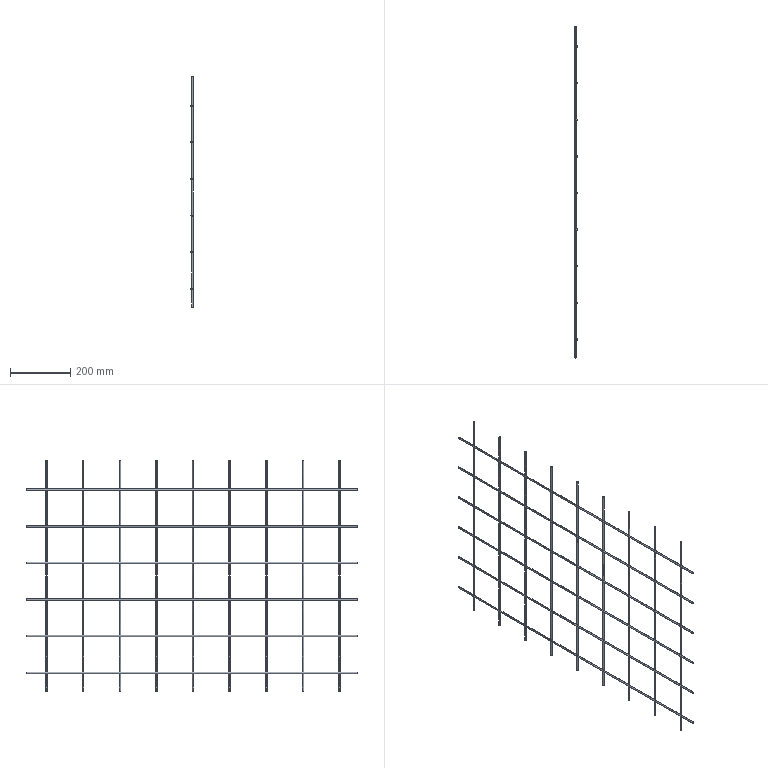Part | 1 solid | 60 faces | box 8 x 1105 x 767 mm | volume 264375 mm3 | cylinder 30 | plane 30 | commonest cylinder face diameters 5 x30